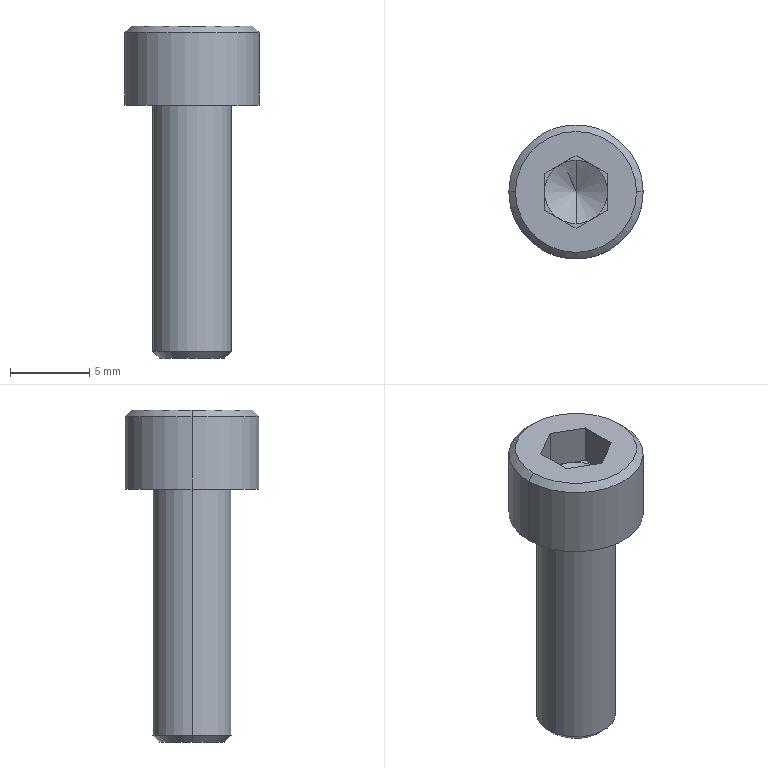Part | SolidWorks | features ICE 2, Chamfer 1, RevCut 1, Revolution 1 | 1 solid | 25 faces | box 8.5 x 8.5 x 21 mm | volume 554.737 mm3 | plane 15 | cone 6 | cylinder 4 | commonest cylinder face diameters 5 x2 8.5 x2
STEP:
#1=CARTESIAN_POINT('',(3.825,0.,5.));
#2=VERTEX_POINT('',#1);
#3=CARTESIAN_POINT('',(-3.825,0.,5.));
#4=VERTEX_POINT('',#3);
#5=CARTESIAN_POINT('',(0.,0.,5.));
#6=DIRECTION('',(0.,0.,1.));
#7=DIRECTION('',(1.,0.,0.));
#8=AXIS2_PLACEMENT_3D('',#5,#6,#7);
#9=CIRCLE('',#8,3.825);
#10=EDGE_CURVE('',#2,#4,#9,.T.);
#11=ORIENTED_EDGE('',*,*,#10,.F.);
#12=CARTESIAN_POINT('',(4.25,0.,4.575));
#13=VERTEX_POINT('',#12);
#14=CARTESIAN_POINT('',(3.825,0.,5.));
#15=DIRECTION('',(0.7071,0.,-0.7071));
#16=VECTOR('',#15,1000.);
#17=LINE('',#14,#16);
#18=EDGE_CURVE('',#2,#13,#17,.T.);
#19=ORIENTED_EDGE('',*,*,#18,.T.);
#20=CARTESIAN_POINT('',(-4.25,0.,4.575));
#21=VERTEX_POINT('',#20);
#22=CARTESIAN_POINT('',(0.,0.,4.575));
#23=DIRECTION('',(0.,0.,-1.));
#24=DIRECTION('',(1.,0.,0.));
#25=AXIS2_PLACEMENT_3D('',#22,#23,#24);
#26=CIRCLE('',#25,4.25);
#27=EDGE_CURVE('',#21,#13,#26,.T.);
#28=ORIENTED_EDGE('',*,*,#27,.F.);
#29=CARTESIAN_POINT('',(-3.825,0.,5.));
#30=DIRECTION('',(-0.7071,0.,-0.7071));
#31=VECTOR('',#30,1000.);
#32=LINE('',#29,#31);
#33=EDGE_CURVE('',#4,#21,#32,.T.);
#34=ORIENTED_EDGE('',*,*,#33,.F.);
#35=EDGE_LOOP('',(#11,#19,#28,#34));
#36=FACE_OUTER_BOUND('',#35,.T.);
#37=CARTESIAN_POINT('',(0.,0.,5.));
#38=DIRECTION('',(0.,0.,-1.));
#39=DIRECTION('',(-1.,0.,0.));
#40=AXIS2_PLACEMENT_3D('',#37,#38,#39);
#41=CONICAL_SURFACE('',#40,3.825,0.7854);
#42=ADVANCED_FACE('',(#36),#41,.T.);
#43=CARTESIAN_POINT('',(-2.075,0.,-16.));
#44=VERTEX_POINT('',#43);
#45=CARTESIAN_POINT('',(2.075,0.,-16.));
#46=VERTEX_POINT('',#45);
#47=CARTESIAN_POINT('',(0.,0.,-16.));
#48=DIRECTION('',(0.,0.,-1.));
#49=DIRECTION('',(-1.,0.,0.));
#50=AXIS2_PLACEMENT_3D('',#47,#48,#49);
#51=CIRCLE('',#50,2.075);
#52=EDGE_CURVE('',#44,#46,#51,.T.);
#53=ORIENTED_EDGE('',*,*,#52,.F.);
#54=CARTESIAN_POINT('',(-2.5,0.,-15.575));
#55=VERTEX_POINT('',#54);
#56=CARTESIAN_POINT('',(-2.075,0.,-16.));
#57=DIRECTION('',(-0.7071,0.,0.7071));
#58=VECTOR('',#57,1000.);
#59=LINE('',#56,#58);
#60=EDGE_CURVE('',#44,#55,#59,.T.);
#61=ORIENTED_EDGE('',*,*,#60,.T.);
#62=CARTESIAN_POINT('',(2.5,0.,-15.575));
#63=VERTEX_POINT('',#62);
#64=CARTESIAN_POINT('',(0.,0.,-15.575));
#65=DIRECTION('',(0.,0.,1.));
#66=DIRECTION('',(-1.,0.,0.));
#67=AXIS2_PLACEMENT_3D('',#64,#65,#66);
#68=CIRCLE('',#67,2.5);
#69=EDGE_CURVE('',#63,#55,#68,.T.);
#70=ORIENTED_EDGE('',*,*,#69,.F.);
#71=CARTESIAN_POINT('',(2.075,0.,-16.));
#72=DIRECTION('',(0.7071,0.,0.7071));
#73=VECTOR('',#72,1000.);
#74=LINE('',#71,#73);
#75=EDGE_CURVE('',#46,#63,#74,.T.);
#76=ORIENTED_EDGE('',*,*,#75,.F.);
#77=EDGE_LOOP('',(#53,#61,#70,#76));
#78=FACE_OUTER_BOUND('',#77,.T.);
#79=CARTESIAN_POINT('',(0.,0.,-16.));
#80=DIRECTION('',(0.,0.,1.));
#81=DIRECTION('',(1.,0.,0.));
#82=AXIS2_PLACEMENT_3D('',#79,#80,#81);
#83=CONICAL_SURFACE('',#82,2.075,0.7854);
#84=ADVANCED_FACE('',(#78),#83,.T.);
#85=CARTESIAN_POINT('',(0.,0.,1.345));
#86=VERTEX_POINT('',#85);
#87=CARTESIAN_POINT('',(0.,-2.,2.5));
#88=VERTEX_POINT('',#87);
#89=CARTESIAN_POINT('',(0.,0.,1.345));
#90=DIRECTION('',(0.,-0.866,0.5));
#91=VECTOR('',#90,1000.);
#92=LINE('',#89,#91);
#93=EDGE_CURVE('',#86,#88,#92,.T.);
#94=ORIENTED_EDGE('',*,*,#93,.F.);
#95=CARTESIAN_POINT('',(0.,2.,2.5));
#96=VERTEX_POINT('',#95);
#97=CARTESIAN_POINT('',(0.,0.,1.345));
#98=DIRECTION('',(0.,0.866,0.5));
#99=VECTOR('',#98,1000.);
#100=LINE('',#97,#99);
#101=EDGE_CURVE('',#86,#96,#100,.T.);
#102=ORIENTED_EDGE('',*,*,#101,.T.);
#103=CARTESIAN_POINT('',(-1.,1.732,2.5));
#104=VERTEX_POINT('',#103);
#105=CARTESIAN_POINT('',(0.,0.,2.5));
#106=DIRECTION('',(0.,0.,-1.));
#107=DIRECTION('',(0.,1.,0.));
#108=AXIS2_PLACEMENT_3D('',#105,#106,#107);
#109=CIRCLE('',#108,2.);
#110=EDGE_CURVE('',#104,#96,#109,.T.);
#111=ORIENTED_EDGE('',*,*,#110,.F.);
#112=CARTESIAN_POINT('',(-2.,0.,2.5));
#113=VERTEX_POINT('',#112);
#114=CARTESIAN_POINT('',(0.,0.,2.5));
#115=DIRECTION('',(0.,0.,-1.));
#116=DIRECTION('',(0.,1.,0.));
#117=AXIS2_PLACEMENT_3D('',#114,#115,#116);
#118=CIRCLE('',#117,2.);
#119=EDGE_CURVE('',#113,#104,#118,.T.);
#120=ORIENTED_EDGE('',*,*,#119,.F.);
#121=CARTESIAN_POINT('',(-1.,-1.732,2.5));
#122=VERTEX_POINT('',#121);
#123=CARTESIAN_POINT('',(0.,0.,2.5));
#124=DIRECTION('',(0.,0.,-1.));
#125=DIRECTION('',(0.,1.,0.));
#126=AXIS2_PLACEMENT_3D('',#123,#124,#125);
#127=CIRCLE('',#126,2.);
#128=EDGE_CURVE('',#122,#113,#127,.T.);
#129=ORIENTED_EDGE('',*,*,#128,.F.);
#130=CARTESIAN_POINT('',(0.,0.,2.5));
#131=DIRECTION('',(0.,0.,-1.));
#132=DIRECTION('',(0.,1.,0.));
#133=AXIS2_PLACEMENT_3D('',#130,#131,#132);
#134=CIRCLE('',#133,2.);
#135=EDGE_CURVE('',#88,#122,#134,.T.);
#136=ORIENTED_EDGE('',*,*,#135,.F.);
#137=EDGE_LOOP('',(#94,#102,#111,#120,#129,#136));
#138=FACE_OUTER_BOUND('',#137,.T.);
#139=CARTESIAN_POINT('',(0.,0.,1001.345));
#140=DIRECTION('',(0.,0.,1.));
#141=DIRECTION('',(0.,-1.,0.));
#142=AXIS2_PLACEMENT_3D('',#139,#140,#141);
#143=CONICAL_SURFACE('',#142,1732.051,1.047);
#144=ADVANCED_FACE('',(#138),#143,.F.);
#145=ORIENTED_EDGE('',*,*,#69,.T.);
#146=CARTESIAN_POINT('',(-2.5,0.,0.));
#147=VERTEX_POINT('',#146);
#148=CARTESIAN_POINT('',(-2.5,0.,-16.));
#149=DIRECTION('',(0.,0.,1.));
#150=VECTOR('',#149,1000.);
#151=LINE('',#148,#150);
#152=EDGE_CURVE('',#55,#147,#151,.T.);
#153=ORIENTED_EDGE('',*,*,#152,.T.);
#154=CARTESIAN_POINT('',(2.5,0.,0.));
#155=VERTEX_POINT('',#154);
#156=CARTESIAN_POINT('',(0.,0.,0.));
#157=DIRECTION('',(0.,0.,-1.));
#158=DIRECTION('',(-1.,0.,0.));
#159=AXIS2_PLACEMENT_3D('',#156,#157,#158);
#160=CIRCLE('',#159,2.5);
#161=EDGE_CURVE('',#147,#155,#160,.T.);
#162=ORIENTED_EDGE('',*,*,#161,.T.);
#163=CARTESIAN_POINT('',(2.5,0.,-16.));
#164=DIRECTION('',(0.,0.,1.));
#165=VECTOR('',#164,1000.);
#166=LINE('',#163,#165);
#167=EDGE_CURVE('',#63,#155,#166,.T.);
#168=ORIENTED_EDGE('',*,*,#167,.F.);
#169=EDGE_LOOP('',(#145,#153,#162,#168));
#170=FACE_OUTER_BOUND('',#169,.T.);
#171=CARTESIAN_POINT('',(0.,0.,-16.));
#172=DIRECTION('',(0.,0.,1.));
#173=DIRECTION('',(1.,0.,0.));
#174=AXIS2_PLACEMENT_3D('',#171,#172,#173);
#175=CYLINDRICAL_SURFACE('',#174,2.5);
#176=ADVANCED_FACE('',(#170),#175,.T.);
#177=CARTESIAN_POINT('',(4.25,0.,0.));
#178=VERTEX_POINT('',#177);
#179=CARTESIAN_POINT('',(-4.25,0.,0.));
#180=VERTEX_POINT('',#179);
#181=CARTESIAN_POINT('',(0.,0.,0.));
#182=DIRECTION('',(0.,0.,1.));
#183=DIRECTION('',(1.,0.,0.));
#184=AXIS2_PLACEMENT_3D('',#181,#182,#183);
#185=CIRCLE('',#184,4.25);
#186=EDGE_CURVE('',#178,#180,#185,.T.);
#187=ORIENTED_EDGE('',*,*,#186,.T.);
#188=CARTESIAN_POINT('',(-4.25,0.,0.));
#189=DIRECTION('',(0.,0.,1.));
#190=VECTOR('',#189,1000.);
#191=LINE('',#188,#190);
#192=EDGE_CURVE('',#180,#21,#191,.T.);
#193=ORIENTED_EDGE('',*,*,#192,.T.);
#194=ORIENTED_EDGE('',*,*,#27,.T.);
#195=CARTESIAN_POINT('',(4.25,0.,0.));
#196=DIRECTION('',(0.,0.,1.));
#197=VECTOR('',#196,1000.);
#198=LINE('',#195,#197);
#199=EDGE_CURVE('',#178,#13,#198,.T.);
#200=ORIENTED_EDGE('',*,*,#199,.F.);
#201=EDGE_LOOP('',(#187,#193,#194,#200));
#202=FACE_OUTER_BOUND('',#201,.T.);
#203=CARTESIAN_POINT('',(0.,0.,0.));
#204=DIRECTION('',(0.,0.,1.));
#205=DIRECTION('',(1.,0.,0.));
#206=AXIS2_PLACEMENT_3D('',#203,#204,#205);
#207=CYLINDRICAL_SURFACE('',#206,4.25);
#208=ADVANCED_FACE('',(#202),#207,.T.);
#209=CARTESIAN_POINT('',(2.,1.155,2.5));
#210=VERTEX_POINT('',#209);
#211=CARTESIAN_POINT('',(1.,1.732,2.5));
#212=VERTEX_POINT('',#211);
#213=CARTESIAN_POINT('',(2.,1.155,2.5));
#214=DIRECTION('',(-0.866,0.5,0.));
#215=VECTOR('',#214,1000.);
#216=LINE('',#213,#215);
#217=EDGE_CURVE('',#210,#212,#216,.T.);
#218=ORIENTED_EDGE('',*,*,#217,.T.);
#219=CARTESIAN_POINT('',(2.,0.,2.5));
#220=VERTEX_POINT('',#219);
#221=CARTESIAN_POINT('',(0.,0.,2.5));
#222=DIRECTION('',(0.,0.,-1.));
#223=DIRECTION('',(0.,1.,0.));
#224=AXIS2_PLACEMENT_3D('',#221,#222,#223);
#225=CIRCLE('',#224,2.);
#226=EDGE_CURVE('',#212,#220,#225,.T.);
#227=ORIENTED_EDGE('',*,*,#226,.T.);
#228=CARTESIAN_POINT('',(2.,-1.155,2.5));
#229=DIRECTION('',(0.,1.,0.));
#230=VECTOR('',#229,1000.);
#231=LINE('',#228,#230);
#232=EDGE_CURVE('',#220,#210,#231,.T.);
#233=ORIENTED_EDGE('',*,*,#232,.T.);
#234=EDGE_LOOP('',(#218,#227,#233));
#235=FACE_OUTER_BOUND('',#234,.T.);
#236=CARTESIAN_POINT('',(0.,0.,2.5));
#237=DIRECTION('',(0.,0.,1.));
#238=DIRECTION('',(1.,0.,0.));
#239=AXIS2_PLACEMENT_3D('',#236,#237,#238);
#240=PLANE('',#239);
#241=ADVANCED_FACE('',(#235),#240,.T.);
#242=CARTESIAN_POINT('',(2.,-1.155,2.5));
#243=VERTEX_POINT('',#242);
#244=CARTESIAN_POINT('',(2.,-1.155,2.5));
#245=DIRECTION('',(0.,1.,0.));
#246=VECTOR('',#245,1000.);
#247=LINE('',#244,#246);
#248=EDGE_CURVE('',#243,#220,#247,.T.);
#249=ORIENTED_EDGE('',*,*,#248,.T.);
#250=CARTESIAN_POINT('',(1.,-1.732,2.5));
#251=VERTEX_POINT('',#250);
#252=CARTESIAN_POINT('',(0.,0.,2.5));
#253=DIRECTION('',(0.,0.,-1.));
#254=DIRECTION('',(0.,1.,0.));
#255=AXIS2_PLACEMENT_3D('',#252,#253,#254);
#256=CIRCLE('',#255,2.);
#257=EDGE_CURVE('',#220,#251,#256,.T.);
#258=ORIENTED_EDGE('',*,*,#257,.T.);
#259=CARTESIAN_POINT('',(0.,-2.309,2.5));
#260=DIRECTION('',(0.866,0.5,0.));
#261=VECTOR('',#260,1000.);
#262=LINE('',#259,#261);
#263=EDGE_CURVE('',#251,#243,#262,.T.);
#264=ORIENTED_EDGE('',*,*,#263,.T.);
#265=EDGE_LOOP('',(#249,#258,#264));
#266=FACE_OUTER_BOUND('',#265,.T.);
#267=CARTESIAN_POINT('',(0.,0.,2.5));
#268=DIRECTION('',(0.,0.,1.));
#269=DIRECTION('',(1.,0.,0.));
#270=AXIS2_PLACEMENT_3D('',#267,#268,#269);
#271=PLANE('',#270);
#272=ADVANCED_FACE('',(#266),#271,.T.);
#273=CARTESIAN_POINT('',(0.,-2.309,2.5));
#274=VERTEX_POINT('',#273);
#275=CARTESIAN_POINT('',(0.,-2.309,2.5));
#276=DIRECTION('',(0.866,0.5,0.));
#277=VECTOR('',#276,1000.);
#278=LINE('',#275,#277);
#279=EDGE_CURVE('',#274,#251,#278,.T.);
#280=ORIENTED_EDGE('',*,*,#279,.T.);
#281=CARTESIAN_POINT('',(0.,0.,2.5));
#282=DIRECTION('',(0.,0.,-1.));
#283=DIRECTION('',(0.,1.,0.));
#284=AXIS2_PLACEMENT_3D('',#281,#282,#283);
#285=CIRCLE('',#284,2.);
#286=EDGE_CURVE('',#251,#88,#285,.T.);
#287=ORIENTED_EDGE('',*,*,#286,.T.);
#288=ORIENTED_EDGE('',*,*,#135,.T.);
#289=CARTESIAN_POINT('',(-2.,-1.155,2.5));
#290=DIRECTION('',(0.866,-0.5,0.));
#291=VECTOR('',#290,1000.);
#292=LINE('',#289,#291);
#293=EDGE_CURVE('',#122,#274,#292,.T.);
#294=ORIENTED_EDGE('',*,*,#293,.T.);
#295=EDGE_LOOP('',(#280,#287,#288,#294));
#296=FACE_OUTER_BOUND('',#295,.T.);
#297=CARTESIAN_POINT('',(0.,0.,2.5));
#298=DIRECTION('',(0.,0.,1.));
#299=DIRECTION('',(1.,0.,0.));
#300=AXIS2_PLACEMENT_3D('',#297,#298,#299);
#301=PLANE('',#300);
#302=ADVANCED_FACE('',(#296),#301,.T.);
#303=CARTESIAN_POINT('',(-2.,-1.155,2.5));
#304=VERTEX_POINT('',#303);
#305=CARTESIAN_POINT('',(-2.,-1.155,2.5));
#306=DIRECTION('',(0.866,-0.5,0.));
#307=VECTOR('',#306,1000.);
#308=LINE('',#305,#307);
#309=EDGE_CURVE('',#304,#122,#308,.T.);
#310=ORIENTED_EDGE('',*,*,#309,.T.);
#311=ORIENTED_EDGE('',*,*,#128,.T.);
#312=CARTESIAN_POINT('',(-2.,1.155,2.5));
#313=DIRECTION('',(0.,-1.,0.));
#314=VECTOR('',#313,1000.);
#315=LINE('',#312,#314);
#316=EDGE_CURVE('',#113,#304,#315,.T.);
#317=ORIENTED_EDGE('',*,*,#316,.T.);
#318=EDGE_LOOP('',(#310,#311,#317));
#319=FACE_OUTER_BOUND('',#318,.T.);
#320=CARTESIAN_POINT('',(0.,0.,2.5));
#321=DIRECTION('',(0.,0.,1.));
#322=DIRECTION('',(1.,0.,0.));
#323=AXIS2_PLACEMENT_3D('',#320,#321,#322);
#324=PLANE('',#323);
#325=ADVANCED_FACE('',(#319),#324,.T.);
#326=CARTESIAN_POINT('',(-2.,1.155,2.5));
#327=VERTEX_POINT('',#326);
#328=CARTESIAN_POINT('',(-2.,1.155,2.5));
#329=DIRECTION('',(0.,-1.,0.));
#330=VECTOR('',#329,1000.);
#331=LINE('',#328,#330);
#332=EDGE_CURVE('',#327,#113,#331,.T.);
#333=ORIENTED_EDGE('',*,*,#332,.T.);
#334=ORIENTED_EDGE('',*,*,#119,.T.);
#335=CARTESIAN_POINT('',(0.,2.309,2.5));
#336=DIRECTION('',(-0.866,-0.5,0.));
#337=VECTOR('',#336,1000.);
#338=LINE('',#335,#337);
#339=EDGE_CURVE('',#104,#327,#338,.T.);
#340=ORIENTED_EDGE('',*,*,#339,.T.);
#341=EDGE_LOOP('',(#333,#334,#340));
#342=FACE_OUTER_BOUND('',#341,.T.);
#343=CARTESIAN_POINT('',(0.,0.,2.5));
#344=DIRECTION('',(0.,0.,1.));
#345=DIRECTION('',(1.,0.,0.));
#346=AXIS2_PLACEMENT_3D('',#343,#344,#345);
#347=PLANE('',#346);
#348=ADVANCED_FACE('',(#342),#347,.T.);
#349=CARTESIAN_POINT('',(0.,2.309,2.5));
#350=VERTEX_POINT('',#349);
#351=CARTESIAN_POINT('',(0.,2.309,2.5));
#352=DIRECTION('',(-0.866,-0.5,0.));
#353=VECTOR('',#352,1000.);
#354=LINE('',#351,#353);
#355=EDGE_CURVE('',#350,#104,#354,.T.);
#356=ORIENTED_EDGE('',*,*,#355,.T.);
#357=ORIENTED_EDGE('',*,*,#110,.T.);
#358=CARTESIAN_POINT('',(0.,0.,2.5));
#359=DIRECTION('',(0.,0.,-1.));
#360=DIRECTION('',(0.,1.,0.));
#361=AXIS2_PLACEMENT_3D('',#358,#359,#360);
#362=CIRCLE('',#361,2.);
#363=EDGE_CURVE('',#96,#212,#362,.T.);
#364=ORIENTED_EDGE('',*,*,#363,.T.);
#365=CARTESIAN_POINT('',(2.,1.155,2.5));
#366=DIRECTION('',(-0.866,0.5,0.));
#367=VECTOR('',#366,1000.);
#368=LINE('',#365,#367);
#369=EDGE_CURVE('',#212,#350,#368,.T.);
#370=ORIENTED_EDGE('',*,*,#369,.T.);
#371=EDGE_LOOP('',(#356,#357,#364,#370));
#372=FACE_OUTER_BOUND('',#371,.T.);
#373=CARTESIAN_POINT('',(0.,0.,2.5));
#374=DIRECTION('',(0.,0.,1.));
#375=DIRECTION('',(1.,0.,0.));
#376=AXIS2_PLACEMENT_3D('',#373,#374,#375);
#377=PLANE('',#376);
#378=ADVANCED_FACE('',(#372),#377,.T.);
#379=ORIENTED_EDGE('',*,*,#186,.F.);
#380=CARTESIAN_POINT('',(0.,0.,0.));
#381=DIRECTION('',(0.,0.,1.));
#382=DIRECTION('',(1.,0.,0.));
#383=AXIS2_PLACEMENT_3D('',#380,#381,#382);
#384=CIRCLE('',#383,4.25);
#385=EDGE_CURVE('',#180,#178,#384,.T.);
#386=ORIENTED_EDGE('',*,*,#385,.F.);
#387=EDGE_LOOP('',(#379,#386));
#388=FACE_OUTER_BOUND('',#387,.T.);
#389=CARTESIAN_POINT('',(0.,0.,0.));
#390=DIRECTION('',(0.,0.,-1.));
#391=DIRECTION('',(-1.,0.,0.));
#392=AXIS2_PLACEMENT_3D('',#389,#390,#391);
#393=CIRCLE('',#392,2.5);
#394=EDGE_CURVE('',#155,#147,#393,.T.);
#395=ORIENTED_EDGE('',*,*,#394,.F.);
#396=ORIENTED_EDGE('',*,*,#161,.F.);
#397=EDGE_LOOP('',(#395,#396));
#398=FACE_BOUND('',#397,.T.);
#399=CARTESIAN_POINT('',(4.25,0.,0.));
#400=DIRECTION('',(0.,0.,-1.));
#401=DIRECTION('',(-1.,0.,0.));
#402=AXIS2_PLACEMENT_3D('',#399,#400,#401);
#403=PLANE('',#402);
#404=ADVANCED_FACE('',(#388,#398),#403,.T.);
#405=ORIENTED_EDGE('',*,*,#192,.F.);
#406=ORIENTED_EDGE('',*,*,#385,.T.);
#407=ORIENTED_EDGE('',*,*,#199,.T.);
#408=CARTESIAN_POINT('',(0.,0.,4.575));
#409=DIRECTION('',(0.,0.,-1.));
#410=DIRECTION('',(1.,0.,0.));
#411=AXIS2_PLACEMENT_3D('',#408,#409,#410);
#412=CIRCLE('',#411,4.25);
#413=EDGE_CURVE('',#13,#21,#412,.T.);
#414=ORIENTED_EDGE('',*,*,#413,.T.);
#415=EDGE_LOOP('',(#405,#406,#407,#414));
#416=FACE_OUTER_BOUND('',#415,.T.);
#417=CARTESIAN_POINT('',(0.,0.,0.));
#418=DIRECTION('',(0.,0.,1.));
#419=DIRECTION('',(1.,0.,0.));
#420=AXIS2_PLACEMENT_3D('',#417,#418,#419);
#421=CYLINDRICAL_SURFACE('',#420,4.25);
#422=ADVANCED_FACE('',(#416),#421,.T.);
#423=CARTESIAN_POINT('',(0.,0.,5.));
#424=DIRECTION('',(0.,0.,1.));
#425=DIRECTION('',(1.,0.,0.));
#426=AXIS2_PLACEMENT_3D('',#423,#424,#425);
#427=CIRCLE('',#426,3.825);
#428=EDGE_CURVE('',#4,#2,#427,.T.);
#429=ORIENTED_EDGE('',*,*,#428,.T.);
#430=ORIENTED_EDGE('',*,*,#10,.T.);
#431=EDGE_LOOP('',(#429,#430));
#432=FACE_OUTER_BOUND('',#431,.T.);
#433=CARTESIAN_POINT('',(2.,-1.155,5.));
#434=VERTEX_POINT('',#433);
#435=CARTESIAN_POINT('',(2.,1.155,5.));
#436=VERTEX_POINT('',#435);
#437=CARTESIAN_POINT('',(2.,-1.155,5.));
#438=DIRECTION('',(0.,1.,0.));
#439=VECTOR('',#438,1000.);
#440=LINE('',#437,#439);
#441=EDGE_CURVE('',#434,#436,#440,.T.);
#442=ORIENTED_EDGE('',*,*,#441,.F.);
#443=CARTESIAN_POINT('',(0.,-2.309,5.));
#444=VERTEX_POINT('',#443);
#445=CARTESIAN_POINT('',(0.,-2.309,5.));
#446=DIRECTION('',(0.866,0.5,0.));
#447=VECTOR('',#446,1000.);
#448=LINE('',#445,#447);
#449=EDGE_CURVE('',#444,#434,#448,.T.);
#450=ORIENTED_EDGE('',*,*,#449,.F.);
#451=CARTESIAN_POINT('',(-2.,-1.155,5.));
#452=VERTEX_POINT('',#451);
#453=CARTESIAN_POINT('',(-2.,-1.155,5.));
#454=DIRECTION('',(0.866,-0.5,0.));
#455=VECTOR('',#454,1000.);
#456=LINE('',#453,#455);
#457=EDGE_CURVE('',#452,#444,#456,.T.);
#458=ORIENTED_EDGE('',*,*,#457,.F.);
#459=CARTESIAN_POINT('',(-2.,1.155,5.));
#460=VERTEX_POINT('',#459);
#461=CARTESIAN_POINT('',(-2.,1.155,5.));
#462=DIRECTION('',(0.,-1.,0.));
#463=VECTOR('',#462,1000.);
#464=LINE('',#461,#463);
#465=EDGE_CURVE('',#460,#452,#464,.T.);
#466=ORIENTED_EDGE('',*,*,#465,.F.);
#467=CARTESIAN_POINT('',(0.,2.309,5.));
#468=VERTEX_POINT('',#467);
#469=CARTESIAN_POINT('',(0.,2.309,5.));
#470=DIRECTION('',(-0.866,-0.5,0.));
#471=VECTOR('',#470,1000.);
#472=LINE('',#469,#471);
#473=EDGE_CURVE('',#468,#460,#472,.T.);
#474=ORIENTED_EDGE('',*,*,#473,.F.);
#475=CARTESIAN_POINT('',(2.,1.155,5.));
#476=DIRECTION('',(-0.866,0.5,0.));
#477=VECTOR('',#476,1000.);
#478=LINE('',#475,#477);
#479=EDGE_CURVE('',#436,#468,#478,.T.);
#480=ORIENTED_EDGE('',*,*,#479,.F.);
#481=EDGE_LOOP('',(#442,#450,#458,#466,#474,#480));
#482=FACE_BOUND('',#481,.T.);
#483=CARTESIAN_POINT('',(0.,0.,5.));
#484=DIRECTION('',(0.,0.,1.));
#485=DIRECTION('',(1.,0.,0.));
#486=AXIS2_PLACEMENT_3D('',#483,#484,#485);
#487=PLANE('',#486);
#488=ADVANCED_FACE('',(#432,#482),#487,.T.);
#489=ORIENTED_EDGE('',*,*,#152,.F.);
#490=CARTESIAN_POINT('',(0.,0.,-15.575));
#491=DIRECTION('',(0.,0.,1.));
#492=DIRECTION('',(-1.,0.,0.));
#493=AXIS2_PLACEMENT_3D('',#490,#491,#492);
#494=CIRCLE('',#493,2.5);
#495=EDGE_CURVE('',#55,#63,#494,.T.);
#496=ORIENTED_EDGE('',*,*,#495,.T.);
#497=ORIENTED_EDGE('',*,*,#167,.T.);
#498=ORIENTED_EDGE('',*,*,#394,.T.);
#499=EDGE_LOOP('',(#489,#496,#497,#498));
#500=FACE_OUTER_BOUND('',#499,.T.);
#501=CARTESIAN_POINT('',(0.,0.,-16.));
#502=DIRECTION('',(0.,0.,1.));
#503=DIRECTION('',(1.,0.,0.));
#504=AXIS2_PLACEMENT_3D('',#501,#502,#503);
#505=CYLINDRICAL_SURFACE('',#504,2.5);
#506=ADVANCED_FACE('',(#500),#505,.T.);
#507=CARTESIAN_POINT('',(0.,0.,-16.));
#508=DIRECTION('',(0.,0.,-1.));
#509=DIRECTION('',(-1.,0.,0.));
#510=AXIS2_PLACEMENT_3D('',#507,#508,#509);
#511=CIRCLE('',#510,2.075);
#512=EDGE_CURVE('',#46,#44,#511,.T.);
#513=ORIENTED_EDGE('',*,*,#512,.T.);
#514=ORIENTED_EDGE('',*,*,#52,.T.);
#515=EDGE_LOOP('',(#513,#514));
#516=FACE_OUTER_BOUND('',#515,.T.);
#517=CARTESIAN_POINT('',(0.,0.,-16.));
#518=DIRECTION('',(0.,0.,-1.));
#519=DIRECTION('',(-1.,0.,0.));
#520=AXIS2_PLACEMENT_3D('',#517,#518,#519);
#521=PLANE('',#520);
#522=ADVANCED_FACE('',(#516),#521,.T.);
#523=ORIENTED_EDGE('',*,*,#441,.T.);
#524=CARTESIAN_POINT('',(2.,1.155,2.5));
#525=DIRECTION('',(0.,0.,1.));
#526=VECTOR('',#525,1000.);
#527=LINE('',#524,#526);
#528=EDGE_CURVE('',#210,#436,#527,.T.);
#529=ORIENTED_EDGE('',*,*,#528,.F.);
#530=ORIENTED_EDGE('',*,*,#232,.F.);
#531=ORIENTED_EDGE('',*,*,#248,.F.);
#532=CARTESIAN_POINT('',(2.,-1.155,2.5));
#533=DIRECTION('',(0.,0.,1.));
#534=VECTOR('',#533,1000.);
#535=LINE('',#532,#534);
#536=EDGE_CURVE('',#243,#434,#535,.T.);
#537=ORIENTED_EDGE('',*,*,#536,.T.);
#538=EDGE_LOOP('',(#523,#529,#530,#531,#537));
#539=FACE_OUTER_BOUND('',#538,.T.);
#540=CARTESIAN_POINT('',(2.,-1.155,2.5));
#541=DIRECTION('',(1.,0.,0.));
#542=DIRECTION('',(0.,0.,-1.));
#543=AXIS2_PLACEMENT_3D('',#540,#541,#542);
#544=PLANE('',#543);
#545=ADVANCED_FACE('',(#539),#544,.F.);
#546=ORIENTED_EDGE('',*,*,#449,.T.);
#547=ORIENTED_EDGE('',*,*,#536,.F.);
#548=ORIENTED_EDGE('',*,*,#263,.F.);
#549=ORIENTED_EDGE('',*,*,#279,.F.);
#550=CARTESIAN_POINT('',(0.,-2.309,2.5));
#551=DIRECTION('',(0.,0.,1.));
#552=VECTOR('',#551,1000.);
#553=LINE('',#550,#552);
#554=EDGE_CURVE('',#274,#444,#553,.T.);
#555=ORIENTED_EDGE('',*,*,#554,.T.);
#556=EDGE_LOOP('',(#546,#547,#548,#549,#555));
#557=FACE_OUTER_BOUND('',#556,.T.);
#558=CARTESIAN_POINT('',(0.,-2.309,2.5));
#559=DIRECTION('',(0.5,-0.866,0.));
#560=DIRECTION('',(0.866,0.5,0.));
#561=AXIS2_PLACEMENT_3D('',#558,#559,#560);
#562=PLANE('',#561);
#563=ADVANCED_FACE('',(#557),#562,.F.);
#564=ORIENTED_EDGE('',*,*,#457,.T.);
#565=ORIENTED_EDGE('',*,*,#554,.F.);
#566=ORIENTED_EDGE('',*,*,#293,.F.);
#567=ORIENTED_EDGE('',*,*,#309,.F.);
#568=CARTESIAN_POINT('',(-2.,-1.155,2.5));
#569=DIRECTION('',(0.,0.,1.));
#570=VECTOR('',#569,1000.);
#571=LINE('',#568,#570);
#572=EDGE_CURVE('',#304,#452,#571,.T.);
#573=ORIENTED_EDGE('',*,*,#572,.T.);
#574=EDGE_LOOP('',(#564,#565,#566,#567,#573));
#575=FACE_OUTER_BOUND('',#574,.T.);
#576=CARTESIAN_POINT('',(-2.,-1.155,2.5));
#577=DIRECTION('',(-0.5,-0.866,0.));
#578=DIRECTION('',(0.866,-0.5,0.));
#579=AXIS2_PLACEMENT_3D('',#576,#577,#578);
#580=PLANE('',#579);
#581=ADVANCED_FACE('',(#575),#580,.F.);
#582=ORIENTED_EDGE('',*,*,#465,.T.);
#583=ORIENTED_EDGE('',*,*,#572,.F.);
#584=ORIENTED_EDGE('',*,*,#316,.F.);
#585=ORIENTED_EDGE('',*,*,#332,.F.);
#586=CARTESIAN_POINT('',(-2.,1.155,2.5));
#587=DIRECTION('',(0.,0.,1.));
#588=VECTOR('',#587,1000.);
#589=LINE('',#586,#588);
#590=EDGE_CURVE('',#327,#460,#589,.T.);
#591=ORIENTED_EDGE('',*,*,#590,.T.);
#592=EDGE_LOOP('',(#582,#583,#584,#585,#591));
#593=FACE_OUTER_BOUND('',#592,.T.);
#594=CARTESIAN_POINT('',(-2.,1.155,2.5));
#595=DIRECTION('',(-1.,0.,0.));
#596=DIRECTION('',(0.,0.,1.));
#597=AXIS2_PLACEMENT_3D('',#594,#595,#596);
#598=PLANE('',#597);
#599=ADVANCED_FACE('',(#593),#598,.F.);
#600=ORIENTED_EDGE('',*,*,#473,.T.);
#601=ORIENTED_EDGE('',*,*,#590,.F.);
#602=ORIENTED_EDGE('',*,*,#339,.F.);
#603=ORIENTED_EDGE('',*,*,#355,.F.);
#604=CARTESIAN_POINT('',(0.,2.309,2.5));
#605=DIRECTION('',(0.,0.,1.));
#606=VECTOR('',#605,1000.);
#607=LINE('',#604,#606);
#608=EDGE_CURVE('',#350,#468,#607,.T.);
#609=ORIENTED_EDGE('',*,*,#608,.T.);
#610=EDGE_LOOP('',(#600,#601,#602,#603,#609));
#611=FACE_OUTER_BOUND('',#610,.T.);
#612=CARTESIAN_POINT('',(0.,2.309,2.5));
#613=DIRECTION('',(-0.5,0.866,0.));
#614=DIRECTION('',(-0.866,-0.5,0.));
#615=AXIS2_PLACEMENT_3D('',#612,#613,#614);
#616=PLANE('',#615);
#617=ADVANCED_FACE('',(#611),#616,.F.);
#618=ORIENTED_EDGE('',*,*,#479,.T.);
#619=ORIENTED_EDGE('',*,*,#608,.F.);
#620=ORIENTED_EDGE('',*,*,#369,.F.);
#621=ORIENTED_EDGE('',*,*,#217,.F.);
#622=ORIENTED_EDGE('',*,*,#528,.T.);
#623=EDGE_LOOP('',(#618,#619,#620,#621,#622));
#624=FACE_OUTER_BOUND('',#623,.T.);
#625=CARTESIAN_POINT('',(2.,1.155,2.5));
#626=DIRECTION('',(0.5,0.866,0.));
#627=DIRECTION('',(-0.866,0.5,0.));
#628=AXIS2_PLACEMENT_3D('',#625,#626,#627);
#629=PLANE('',#628);
#630=ADVANCED_FACE('',(#624),#629,.F.);
#631=ORIENTED_EDGE('',*,*,#101,.F.);
#632=ORIENTED_EDGE('',*,*,#93,.T.);
#633=ORIENTED_EDGE('',*,*,#286,.F.);
#634=ORIENTED_EDGE('',*,*,#257,.F.);
#635=ORIENTED_EDGE('',*,*,#226,.F.);
#636=ORIENTED_EDGE('',*,*,#363,.F.);
#637=EDGE_LOOP('',(#631,#632,#633,#634,#635,#636));
#638=FACE_OUTER_BOUND('',#637,.T.);
#639=CARTESIAN_POINT('',(0.,0.,1001.345));
#640=DIRECTION('',(0.,0.,1.));
#641=DIRECTION('',(0.,-1.,0.));
#642=AXIS2_PLACEMENT_3D('',#639,#640,#641);
#643=CONICAL_SURFACE('',#642,1732.051,1.047);
#644=ADVANCED_FACE('',(#638),#643,.F.);
#645=ORIENTED_EDGE('',*,*,#60,.F.);
#646=ORIENTED_EDGE('',*,*,#512,.F.);
#647=ORIENTED_EDGE('',*,*,#75,.T.);
#648=ORIENTED_EDGE('',*,*,#495,.F.);
#649=EDGE_LOOP('',(#645,#646,#647,#648));
#650=FACE_OUTER_BOUND('',#649,.T.);
#651=CARTESIAN_POINT('',(0.,0.,-16.));
#652=DIRECTION('',(0.,0.,1.));
#653=DIRECTION('',(1.,0.,0.));
#654=AXIS2_PLACEMENT_3D('',#651,#652,#653);
#655=CONICAL_SURFACE('',#654,2.075,0.7854);
#656=ADVANCED_FACE('',(#650),#655,.T.);
#657=ORIENTED_EDGE('',*,*,#18,.F.);
#658=ORIENTED_EDGE('',*,*,#428,.F.);
#659=ORIENTED_EDGE('',*,*,#33,.T.);
#660=ORIENTED_EDGE('',*,*,#413,.F.);
#661=EDGE_LOOP('',(#657,#658,#659,#660));
#662=FACE_OUTER_BOUND('',#661,.T.);
#663=CARTESIAN_POINT('',(0.,0.,5.));
#664=DIRECTION('',(0.,0.,-1.));
#665=DIRECTION('',(-1.,0.,0.));
#666=AXIS2_PLACEMENT_3D('',#663,#664,#665);
#667=CONICAL_SURFACE('',#666,3.825,0.7854);
#668=ADVANCED_FACE('',(#662),#667,.T.);
#669=CLOSED_SHELL('',(#42,#84,#144,#176,#208,#241,#272,#302,#325,#348,#378,#404,#422,#488,#506,#522,#545,#563,#581,#599,#617,#630,#644,#656,#668));
#670=MANIFOLD_SOLID_BREP('',#669);
#671=CARTESIAN_POINT('',(0.,0.,0.));
#672=DIRECTION('',(0.,0.,1.));
#673=DIRECTION('',(1.,0.,0.));
#674=AXIS2_PLACEMENT_3D('',#671,#672,#673);
#675=(LENGTH_UNIT()NAMED_UNIT(*)SI_UNIT(.MILLI.,.METRE.));
#676=UNCERTAINTY_MEASURE_WITH_UNIT(LENGTH_MEASURE(0.00001),#675,'','');
#677=(NAMED_UNIT(*)PLANE_ANGLE_UNIT()SI_UNIT($,.RADIAN.));
#678=(NAMED_UNIT(*)SI_UNIT($,.STERADIAN.)SOLID_ANGLE_UNIT());
#679=(GEOMETRIC_REPRESENTATION_CONTEXT(3)GLOBAL_UNCERTAINTY_ASSIGNED_CONTEXT((#676))GLOBAL_UNIT_ASSIGNED_CONTEXT((#675,#677,#678))REPRESENTATION_CONTEXT('',''));
#680=ADVANCED_BREP_SHAPE_REPRESENTATION('',(#670,#674),#679);